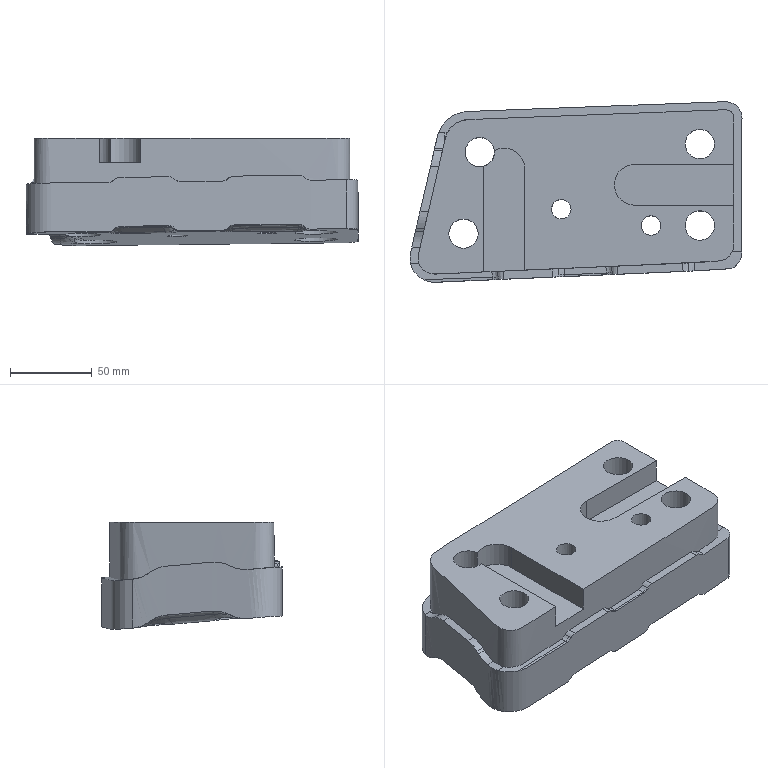Part | NX | features solid 2 | 1 solid | 120 faces | box 203.739 x 110.79 x 65.763 mm | volume 934468 mm3 | spline 96 | cylinder 13 | plane 11 | commonest cylinder face diameters 18 x4 26 x4 25 x3 12 x2